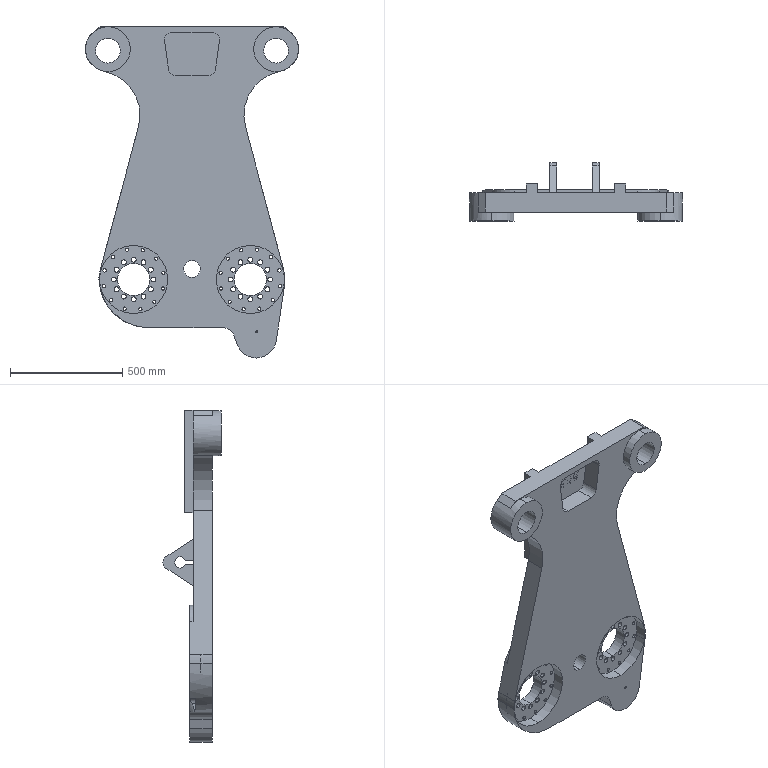Part | SolidWorks | features ICE 19, Fillet 4, HoleWzd 2, Extrusion 1, SweepCut 1 | 2 solids | 867 faces | box 949.998 x 259.953 x 1480 mm | volume 71064561 mm3 | plane 404 | cylinder 233 | spline 176 | cone 50 | torus 4 | commonest cylinder face diameters 22 x50 14.5 x48 25 x48 12 x24 105 x8 132 x8